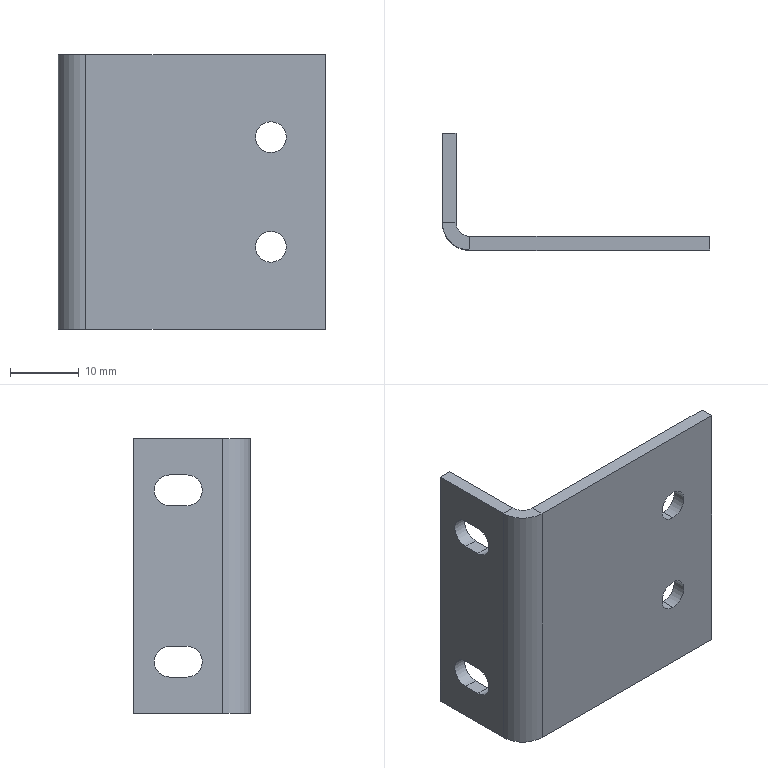Part | SolidWorks | features HoleWzd 2, FlatPattern 1, SMBaseFlange 1, SheetMetal 1 | 1 solid | 26 faces | box 39 x 17 x 40 mm | volume 4045 mm3 | plane 16 | cylinder 10 | commonest cylinder face diameters 4.5 x8 4 x1 8 x1
STEP:
#1=CARTESIAN_POINT('',(31.,-17.,9.75));
#2=VERTEX_POINT('',#1);
#3=CARTESIAN_POINT('',(31.,-17.,14.25));
#4=VERTEX_POINT('',#3);
#5=CARTESIAN_POINT('',(31.,-17.,12.));
#6=DIRECTION('',(0.,1.,0.));
#7=DIRECTION('',(0.,0.,1.));
#8=AXIS2_PLACEMENT_3D('',#5,#6,#7);
#9=CIRCLE('',#8,2.25);
#10=EDGE_CURVE('',#2,#4,#9,.T.);
#11=ORIENTED_EDGE('',*,*,#10,.F.);
#12=CARTESIAN_POINT('',(31.,-15.,9.75));
#13=VERTEX_POINT('',#12);
#14=CARTESIAN_POINT('',(31.,-15.,9.75));
#15=DIRECTION('',(0.,1.,0.));
#16=VECTOR('',#15,1000.);
#17=LINE('',#14,#16);
#18=EDGE_CURVE('',#2,#13,#17,.T.);
#19=ORIENTED_EDGE('',*,*,#18,.T.);
#20=CARTESIAN_POINT('',(31.,-15.,14.25));
#21=VERTEX_POINT('',#20);
#22=CARTESIAN_POINT('',(31.,-15.,12.));
#23=DIRECTION('',(0.,1.,0.));
#24=DIRECTION('',(0.,0.,1.));
#25=AXIS2_PLACEMENT_3D('',#22,#23,#24);
#26=CIRCLE('',#25,2.25);
#27=EDGE_CURVE('',#13,#21,#26,.T.);
#28=ORIENTED_EDGE('',*,*,#27,.T.);
#29=CARTESIAN_POINT('',(31.,-15.,14.25));
#30=DIRECTION('',(0.,1.,0.));
#31=VECTOR('',#30,1000.);
#32=LINE('',#29,#31);
#33=EDGE_CURVE('',#4,#21,#32,.T.);
#34=ORIENTED_EDGE('',*,*,#33,.F.);
#35=EDGE_LOOP('',(#11,#19,#28,#34));
#36=FACE_OUTER_BOUND('',#35,.T.);
#37=CARTESIAN_POINT('',(31.,-15.,12.));
#38=DIRECTION('',(0.,1.,0.));
#39=DIRECTION('',(0.,0.,1.));
#40=AXIS2_PLACEMENT_3D('',#37,#38,#39);
#41=CYLINDRICAL_SURFACE('',#40,2.25);
#42=ADVANCED_FACE('',(#36),#41,.F.);
#43=CARTESIAN_POINT('',(31.,-17.,25.75));
#44=VERTEX_POINT('',#43);
#45=CARTESIAN_POINT('',(31.,-17.,30.25));
#46=VERTEX_POINT('',#45);
#47=CARTESIAN_POINT('',(31.,-17.,28.));
#48=DIRECTION('',(0.,1.,0.));
#49=DIRECTION('',(0.,0.,1.));
#50=AXIS2_PLACEMENT_3D('',#47,#48,#49);
#51=CIRCLE('',#50,2.25);
#52=EDGE_CURVE('',#44,#46,#51,.T.);
#53=ORIENTED_EDGE('',*,*,#52,.F.);
#54=CARTESIAN_POINT('',(31.,-15.,25.75));
#55=VERTEX_POINT('',#54);
#56=CARTESIAN_POINT('',(31.,-15.,25.75));
#57=DIRECTION('',(0.,1.,0.));
#58=VECTOR('',#57,1000.);
#59=LINE('',#56,#58);
#60=EDGE_CURVE('',#44,#55,#59,.T.);
#61=ORIENTED_EDGE('',*,*,#60,.T.);
#62=CARTESIAN_POINT('',(31.,-15.,30.25));
#63=VERTEX_POINT('',#62);
#64=CARTESIAN_POINT('',(31.,-15.,28.));
#65=DIRECTION('',(0.,1.,0.));
#66=DIRECTION('',(0.,0.,1.));
#67=AXIS2_PLACEMENT_3D('',#64,#65,#66);
#68=CIRCLE('',#67,2.25);
#69=EDGE_CURVE('',#55,#63,#68,.T.);
#70=ORIENTED_EDGE('',*,*,#69,.T.);
#71=CARTESIAN_POINT('',(31.,-15.,30.25));
#72=DIRECTION('',(0.,1.,0.));
#73=VECTOR('',#72,1000.);
#74=LINE('',#71,#73);
#75=EDGE_CURVE('',#46,#63,#74,.T.);
#76=ORIENTED_EDGE('',*,*,#75,.F.);
#77=EDGE_LOOP('',(#53,#61,#70,#76));
#78=FACE_OUTER_BOUND('',#77,.T.);
#79=CARTESIAN_POINT('',(31.,-15.,28.));
#80=DIRECTION('',(0.,1.,0.));
#81=DIRECTION('',(0.,0.,1.));
#82=AXIS2_PLACEMENT_3D('',#79,#80,#81);
#83=CYLINDRICAL_SURFACE('',#82,2.25);
#84=ADVANCED_FACE('',(#78),#83,.F.);
#85=CARTESIAN_POINT('',(0.,-13.,40.));
#86=VERTEX_POINT('',#85);
#87=CARTESIAN_POINT('',(2.,-13.,40.));
#88=VERTEX_POINT('',#87);
#89=CARTESIAN_POINT('',(0.,-13.,40.));
#90=DIRECTION('',(1.,0.,0.));
#91=VECTOR('',#90,1000.);
#92=LINE('',#89,#91);
#93=EDGE_CURVE('',#86,#88,#92,.T.);
#94=ORIENTED_EDGE('',*,*,#93,.F.);
#95=CARTESIAN_POINT('',(4.,-17.,40.));
#96=VERTEX_POINT('',#95);
#97=CARTESIAN_POINT('',(4.,-13.,40.));
#98=DIRECTION('',(0.,0.,1.));
#99=DIRECTION('',(-1.,0.,0.));
#100=AXIS2_PLACEMENT_3D('',#97,#98,#99);
#101=CIRCLE('',#100,4.);
#102=EDGE_CURVE('',#86,#96,#101,.T.);
#103=ORIENTED_EDGE('',*,*,#102,.T.);
#104=CARTESIAN_POINT('',(4.,-15.,40.));
#105=VERTEX_POINT('',#104);
#106=CARTESIAN_POINT('',(4.,-15.,40.));
#107=DIRECTION('',(0.,-1.,0.));
#108=VECTOR('',#107,1000.);
#109=LINE('',#106,#108);
#110=EDGE_CURVE('',#105,#96,#109,.T.);
#111=ORIENTED_EDGE('',*,*,#110,.F.);
#112=CARTESIAN_POINT('',(4.,-13.,40.));
#113=DIRECTION('',(0.,0.,1.));
#114=DIRECTION('',(1.,0.,0.));
#115=AXIS2_PLACEMENT_3D('',#112,#113,#114);
#116=CIRCLE('',#115,2.);
#117=EDGE_CURVE('',#88,#105,#116,.T.);
#118=ORIENTED_EDGE('',*,*,#117,.F.);
#119=EDGE_LOOP('',(#94,#103,#111,#118));
#120=FACE_OUTER_BOUND('',#119,.T.);
#121=CARTESIAN_POINT('',(0.,-13.,40.));
#122=DIRECTION('',(0.,0.,1.));
#123=DIRECTION('',(1.,0.,0.));
#124=AXIS2_PLACEMENT_3D('',#121,#122,#123);
#125=PLANE('',#124);
#126=ADVANCED_FACE('',(#120),#125,.T.);
#127=CARTESIAN_POINT('',(0.,0.,40.));
#128=VERTEX_POINT('',#127);
#129=CARTESIAN_POINT('',(0.,0.,40.));
#130=DIRECTION('',(0.,-1.,0.));
#131=VECTOR('',#130,1000.);
#132=LINE('',#129,#131);
#133=EDGE_CURVE('',#128,#86,#132,.T.);
#134=ORIENTED_EDGE('',*,*,#133,.T.);
#135=ORIENTED_EDGE('',*,*,#93,.T.);
#136=CARTESIAN_POINT('',(2.,0.,40.));
#137=VERTEX_POINT('',#136);
#138=CARTESIAN_POINT('',(2.,0.,40.));
#139=DIRECTION('',(0.,-1.,0.));
#140=VECTOR('',#139,1000.);
#141=LINE('',#138,#140);
#142=EDGE_CURVE('',#137,#88,#141,.T.);
#143=ORIENTED_EDGE('',*,*,#142,.F.);
#144=CARTESIAN_POINT('',(0.,0.,40.));
#145=DIRECTION('',(1.,0.,0.));
#146=VECTOR('',#145,1000.);
#147=LINE('',#144,#146);
#148=EDGE_CURVE('',#128,#137,#147,.T.);
#149=ORIENTED_EDGE('',*,*,#148,.F.);
#150=EDGE_LOOP('',(#134,#135,#143,#149));
#151=FACE_OUTER_BOUND('',#150,.T.);
#152=CARTESIAN_POINT('',(4.,-15.,40.));
#153=DIRECTION('',(0.,0.,1.));
#154=DIRECTION('',(1.,0.,0.));
#155=AXIS2_PLACEMENT_3D('',#152,#153,#154);
#156=PLANE('',#155);
#157=ADVANCED_FACE('',(#151),#156,.T.);
#158=CARTESIAN_POINT('',(4.,-17.,0.));
#159=VERTEX_POINT('',#158);
#160=CARTESIAN_POINT('',(4.,-15.,0.));
#161=VERTEX_POINT('',#160);
#162=CARTESIAN_POINT('',(4.,-17.,0.));
#163=DIRECTION('',(0.,1.,0.));
#164=VECTOR('',#163,1000.);
#165=LINE('',#162,#164);
#166=EDGE_CURVE('',#159,#161,#165,.T.);
#167=ORIENTED_EDGE('',*,*,#166,.F.);
#168=CARTESIAN_POINT('',(0.,-13.,0.));
#169=VERTEX_POINT('',#168);
#170=CARTESIAN_POINT('',(4.,-13.,0.));
#171=DIRECTION('',(0.,0.,1.));
#172=DIRECTION('',(-1.,0.,0.));
#173=AXIS2_PLACEMENT_3D('',#170,#171,#172);
#174=CIRCLE('',#173,4.);
#175=EDGE_CURVE('',#169,#159,#174,.T.);
#176=ORIENTED_EDGE('',*,*,#175,.F.);
#177=CARTESIAN_POINT('',(2.,-13.,0.));
#178=VERTEX_POINT('',#177);
#179=CARTESIAN_POINT('',(2.,-13.,0.));
#180=DIRECTION('',(-1.,0.,0.));
#181=VECTOR('',#180,1000.);
#182=LINE('',#179,#181);
#183=EDGE_CURVE('',#178,#169,#182,.T.);
#184=ORIENTED_EDGE('',*,*,#183,.F.);
#185=CARTESIAN_POINT('',(4.,-13.,0.));
#186=DIRECTION('',(0.,0.,1.));
#187=DIRECTION('',(1.,0.,0.));
#188=AXIS2_PLACEMENT_3D('',#185,#186,#187);
#189=CIRCLE('',#188,2.);
#190=EDGE_CURVE('',#178,#161,#189,.T.);
#191=ORIENTED_EDGE('',*,*,#190,.T.);
#192=EDGE_LOOP('',(#167,#176,#184,#191));
#193=FACE_OUTER_BOUND('',#192,.T.);
#194=CARTESIAN_POINT('',(4.,-17.,0.));
#195=DIRECTION('',(0.,0.,-1.));
#196=DIRECTION('',(-1.,0.,0.));
#197=AXIS2_PLACEMENT_3D('',#194,#195,#196);
#198=PLANE('',#197);
#199=ADVANCED_FACE('',(#193),#198,.T.);
#200=CARTESIAN_POINT('',(39.,-17.,0.));
#201=VERTEX_POINT('',#200);
#202=CARTESIAN_POINT('',(0.,-17.,0.));
#203=DIRECTION('',(1.,0.,0.));
#204=VECTOR('',#203,1000.);
#205=LINE('',#202,#204);
#206=EDGE_CURVE('',#159,#201,#205,.T.);
#207=ORIENTED_EDGE('',*,*,#206,.F.);
#208=ORIENTED_EDGE('',*,*,#166,.T.);
#209=CARTESIAN_POINT('',(39.,-15.,0.));
#210=VERTEX_POINT('',#209);
#211=CARTESIAN_POINT('',(0.,-15.,0.));
#212=DIRECTION('',(1.,0.,0.));
#213=VECTOR('',#212,1000.);
#214=LINE('',#211,#213);
#215=EDGE_CURVE('',#161,#210,#214,.T.);
#216=ORIENTED_EDGE('',*,*,#215,.T.);
#217=CARTESIAN_POINT('',(39.,-15.,0.));
#218=DIRECTION('',(0.,-1.,0.));
#219=VECTOR('',#218,1000.);
#220=LINE('',#217,#219);
#221=EDGE_CURVE('',#210,#201,#220,.T.);
#222=ORIENTED_EDGE('',*,*,#221,.T.);
#223=EDGE_LOOP('',(#207,#208,#216,#222));
#224=FACE_OUTER_BOUND('',#223,.T.);
#225=CARTESIAN_POINT('',(2.,-13.,0.));
#226=DIRECTION('',(0.,0.,-1.));
#227=DIRECTION('',(-1.,0.,0.));
#228=AXIS2_PLACEMENT_3D('',#225,#226,#227);
#229=PLANE('',#228);
#230=ADVANCED_FACE('',(#224),#229,.T.);
#231=CARTESIAN_POINT('',(31.,-17.,12.));
#232=DIRECTION('',(0.,1.,0.));
#233=DIRECTION('',(0.,0.,1.));
#234=AXIS2_PLACEMENT_3D('',#231,#232,#233);
#235=CIRCLE('',#234,2.25);
#236=EDGE_CURVE('',#4,#2,#235,.T.);
#237=ORIENTED_EDGE('',*,*,#236,.T.);
#238=ORIENTED_EDGE('',*,*,#10,.T.);
#239=EDGE_LOOP('',(#237,#238));
#240=FACE_BOUND('',#239,.T.);
#241=CARTESIAN_POINT('',(31.,-17.,28.));
#242=DIRECTION('',(0.,1.,0.));
#243=DIRECTION('',(0.,0.,1.));
#244=AXIS2_PLACEMENT_3D('',#241,#242,#243);
#245=CIRCLE('',#244,2.25);
#246=EDGE_CURVE('',#46,#44,#245,.T.);
#247=ORIENTED_EDGE('',*,*,#246,.T.);
#248=ORIENTED_EDGE('',*,*,#52,.T.);
#249=EDGE_LOOP('',(#247,#248));
#250=FACE_BOUND('',#249,.T.);
#251=ORIENTED_EDGE('',*,*,#206,.T.);
#252=CARTESIAN_POINT('',(39.,-17.,40.));
#253=VERTEX_POINT('',#252);
#254=CARTESIAN_POINT('',(39.,-17.,40.));
#255=DIRECTION('',(0.,0.,-1.));
#256=VECTOR('',#255,1000.);
#257=LINE('',#254,#256);
#258=EDGE_CURVE('',#253,#201,#257,.T.);
#259=ORIENTED_EDGE('',*,*,#258,.F.);
#260=CARTESIAN_POINT('',(0.,-17.,40.));
#261=DIRECTION('',(1.,0.,0.));
#262=VECTOR('',#261,1000.);
#263=LINE('',#260,#262);
#264=EDGE_CURVE('',#96,#253,#263,.T.);
#265=ORIENTED_EDGE('',*,*,#264,.F.);
#266=CARTESIAN_POINT('',(4.,-17.,40.));
#267=DIRECTION('',(0.,0.,-1.));
#268=VECTOR('',#267,1000.);
#269=LINE('',#266,#268);
#270=EDGE_CURVE('',#96,#159,#269,.T.);
#271=ORIENTED_EDGE('',*,*,#270,.T.);
#272=EDGE_LOOP('',(#251,#259,#265,#271));
#273=FACE_OUTER_BOUND('',#272,.T.);
#274=CARTESIAN_POINT('',(0.,-17.,40.));
#275=DIRECTION('',(0.,1.,0.));
#276=DIRECTION('',(0.,0.,1.));
#277=AXIS2_PLACEMENT_3D('',#274,#275,#276);
#278=PLANE('',#277);
#279=ADVANCED_FACE('',(#240,#250,#273),#278,.F.);
#280=ORIENTED_EDGE('',*,*,#221,.F.);
#281=CARTESIAN_POINT('',(39.,-15.,40.));
#282=VERTEX_POINT('',#281);
#283=CARTESIAN_POINT('',(39.,-15.,40.));
#284=DIRECTION('',(0.,0.,-1.));
#285=VECTOR('',#284,1000.);
#286=LINE('',#283,#285);
#287=EDGE_CURVE('',#282,#210,#286,.T.);
#288=ORIENTED_EDGE('',*,*,#287,.F.);
#289=CARTESIAN_POINT('',(39.,-15.,40.));
#290=DIRECTION('',(0.,-1.,0.));
#291=VECTOR('',#290,1000.);
#292=LINE('',#289,#291);
#293=EDGE_CURVE('',#282,#253,#292,.T.);
#294=ORIENTED_EDGE('',*,*,#293,.T.);
#295=ORIENTED_EDGE('',*,*,#258,.T.);
#296=EDGE_LOOP('',(#280,#288,#294,#295));
#297=FACE_OUTER_BOUND('',#296,.T.);
#298=CARTESIAN_POINT('',(39.,-15.,40.));
#299=DIRECTION('',(1.,0.,0.));
#300=DIRECTION('',(0.,0.,-1.));
#301=AXIS2_PLACEMENT_3D('',#298,#299,#300);
#302=PLANE('',#301);
#303=ADVANCED_FACE('',(#297),#302,.T.);
#304=CARTESIAN_POINT('',(31.,-15.,12.));
#305=DIRECTION('',(0.,1.,0.));
#306=DIRECTION('',(0.,0.,1.));
#307=AXIS2_PLACEMENT_3D('',#304,#305,#306);
#308=CIRCLE('',#307,2.25);
#309=EDGE_CURVE('',#21,#13,#308,.T.);
#310=ORIENTED_EDGE('',*,*,#309,.F.);
#311=ORIENTED_EDGE('',*,*,#27,.F.);
#312=EDGE_LOOP('',(#310,#311));
#313=FACE_BOUND('',#312,.T.);
#314=CARTESIAN_POINT('',(31.,-15.,28.));
#315=DIRECTION('',(0.,1.,0.));
#316=DIRECTION('',(0.,0.,1.));
#317=AXIS2_PLACEMENT_3D('',#314,#315,#316);
#318=CIRCLE('',#317,2.25);
#319=EDGE_CURVE('',#63,#55,#318,.T.);
#320=ORIENTED_EDGE('',*,*,#319,.F.);
#321=ORIENTED_EDGE('',*,*,#69,.F.);
#322=EDGE_LOOP('',(#320,#321));
#323=FACE_BOUND('',#322,.T.);
#324=ORIENTED_EDGE('',*,*,#215,.F.);
#325=CARTESIAN_POINT('',(4.,-15.,40.));
#326=DIRECTION('',(0.,0.,-1.));
#327=VECTOR('',#326,1000.);
#328=LINE('',#325,#327);
#329=EDGE_CURVE('',#105,#161,#328,.T.);
#330=ORIENTED_EDGE('',*,*,#329,.F.);
#331=CARTESIAN_POINT('',(0.,-15.,40.));
#332=DIRECTION('',(1.,0.,0.));
#333=VECTOR('',#332,1000.);
#334=LINE('',#331,#333);
#335=EDGE_CURVE('',#105,#282,#334,.T.);
#336=ORIENTED_EDGE('',*,*,#335,.T.);
#337=ORIENTED_EDGE('',*,*,#287,.T.);
#338=EDGE_LOOP('',(#324,#330,#336,#337));
#339=FACE_OUTER_BOUND('',#338,.T.);
#340=CARTESIAN_POINT('',(0.,-15.,40.));
#341=DIRECTION('',(0.,1.,0.));
#342=DIRECTION('',(0.,0.,1.));
#343=AXIS2_PLACEMENT_3D('',#340,#341,#342);
#344=PLANE('',#343);
#345=ADVANCED_FACE('',(#313,#323,#339),#344,.T.);
#346=ORIENTED_EDGE('',*,*,#190,.F.);
#347=CARTESIAN_POINT('',(2.,-13.,40.));
#348=DIRECTION('',(0.,0.,-1.));
#349=VECTOR('',#348,1000.);
#350=LINE('',#347,#349);
#351=EDGE_CURVE('',#88,#178,#350,.T.);
#352=ORIENTED_EDGE('',*,*,#351,.F.);
#353=ORIENTED_EDGE('',*,*,#117,.T.);
#354=ORIENTED_EDGE('',*,*,#329,.T.);
#355=EDGE_LOOP('',(#346,#352,#353,#354));
#356=FACE_OUTER_BOUND('',#355,.T.);
#357=CARTESIAN_POINT('',(4.,-13.,40.));
#358=DIRECTION('',(0.,0.,-1.));
#359=DIRECTION('',(-1.,0.,0.));
#360=AXIS2_PLACEMENT_3D('',#357,#358,#359);
#361=CYLINDRICAL_SURFACE('',#360,2.);
#362=ADVANCED_FACE('',(#356),#361,.F.);
#363=CARTESIAN_POINT('',(2.,-7.75,5.25));
#364=VERTEX_POINT('',#363);
#365=CARTESIAN_POINT('',(2.,-5.25,5.25));
#366=VERTEX_POINT('',#365);
#367=CARTESIAN_POINT('',(2.,-7.75,5.25));
#368=DIRECTION('',(0.,1.,0.));
#369=VECTOR('',#368,1000.);
#370=LINE('',#367,#369);
#371=EDGE_CURVE('',#364,#366,#370,.T.);
#372=ORIENTED_EDGE('',*,*,#371,.F.);
#373=CARTESIAN_POINT('',(2.,-7.75,9.75));
#374=VERTEX_POINT('',#373);
#375=CARTESIAN_POINT('',(2.,-7.75,7.5));
#376=DIRECTION('',(1.,0.,0.));
#377=DIRECTION('',(0.,0.,-1.));
#378=AXIS2_PLACEMENT_3D('',#375,#376,#377);
#379=CIRCLE('',#378,2.25);
#380=EDGE_CURVE('',#374,#364,#379,.T.);
#381=ORIENTED_EDGE('',*,*,#380,.F.);
#382=CARTESIAN_POINT('',(2.,-5.25,9.75));
#383=VERTEX_POINT('',#382);
#384=CARTESIAN_POINT('',(2.,-7.75,9.75));
#385=DIRECTION('',(0.,1.,0.));
#386=VECTOR('',#385,1000.);
#387=LINE('',#384,#386);
#388=EDGE_CURVE('',#374,#383,#387,.T.);
#389=ORIENTED_EDGE('',*,*,#388,.T.);
#390=CARTESIAN_POINT('',(2.,-5.25,7.5));
#391=DIRECTION('',(1.,0.,0.));
#392=DIRECTION('',(0.,0.,-1.));
#393=AXIS2_PLACEMENT_3D('',#390,#391,#392);
#394=CIRCLE('',#393,2.25);
#395=EDGE_CURVE('',#366,#383,#394,.T.);
#396=ORIENTED_EDGE('',*,*,#395,.F.);
#397=EDGE_LOOP('',(#372,#381,#389,#396));
#398=FACE_BOUND('',#397,.T.);
#399=CARTESIAN_POINT('',(2.,-5.25,30.25));
#400=VERTEX_POINT('',#399);
#401=CARTESIAN_POINT('',(2.,-5.25,34.75));
#402=VERTEX_POINT('',#401);
#403=CARTESIAN_POINT('',(2.,-5.25,32.5));
#404=DIRECTION('',(1.,0.,0.));
#405=DIRECTION('',(0.,0.,-1.));
#406=AXIS2_PLACEMENT_3D('',#403,#404,#405);
#407=CIRCLE('',#406,2.25);
#408=EDGE_CURVE('',#400,#402,#407,.T.);
#409=ORIENTED_EDGE('',*,*,#408,.F.);
#410=CARTESIAN_POINT('',(2.,-7.75,30.25));
#411=VERTEX_POINT('',#410);
#412=CARTESIAN_POINT('',(2.,-7.75,30.25));
#413=DIRECTION('',(0.,1.,0.));
#414=VECTOR('',#413,1000.);
#415=LINE('',#412,#414);
#416=EDGE_CURVE('',#411,#400,#415,.T.);
#417=ORIENTED_EDGE('',*,*,#416,.F.);
#418=CARTESIAN_POINT('',(2.,-7.75,34.75));
#419=VERTEX_POINT('',#418);
#420=CARTESIAN_POINT('',(2.,-7.75,32.5));
#421=DIRECTION('',(1.,0.,0.));
#422=DIRECTION('',(0.,0.,-1.));
#423=AXIS2_PLACEMENT_3D('',#420,#421,#422);
#424=CIRCLE('',#423,2.25);
#425=EDGE_CURVE('',#419,#411,#424,.T.);
#426=ORIENTED_EDGE('',*,*,#425,.F.);
#427=CARTESIAN_POINT('',(2.,-7.75,34.75));
#428=DIRECTION('',(0.,1.,0.));
#429=VECTOR('',#428,1000.);
#430=LINE('',#427,#429);
#431=EDGE_CURVE('',#419,#402,#430,.T.);
#432=ORIENTED_EDGE('',*,*,#431,.T.);
#433=EDGE_LOOP('',(#409,#417,#426,#432));
#434=FACE_BOUND('',#433,.T.);
#435=CARTESIAN_POINT('',(2.,0.,0.));
#436=VERTEX_POINT('',#435);
#437=CARTESIAN_POINT('',(2.,0.,0.));
#438=DIRECTION('',(0.,-1.,0.));
#439=VECTOR('',#438,1000.);
#440=LINE('',#437,#439);
#441=EDGE_CURVE('',#436,#178,#440,.T.);
#442=ORIENTED_EDGE('',*,*,#441,.F.);
#443=CARTESIAN_POINT('',(2.,0.,40.));
#444=DIRECTION('',(0.,0.,-1.));
#445=VECTOR('',#444,1000.);
#446=LINE('',#443,#445);
#447=EDGE_CURVE('',#137,#436,#446,.T.);
#448=ORIENTED_EDGE('',*,*,#447,.F.);
#449=ORIENTED_EDGE('',*,*,#142,.T.);
#450=ORIENTED_EDGE('',*,*,#351,.T.);
#451=EDGE_LOOP('',(#442,#448,#449,#450));
#452=FACE_OUTER_BOUND('',#451,.T.);
#453=CARTESIAN_POINT('',(2.,0.,40.));
#454=DIRECTION('',(1.,0.,0.));
#455=DIRECTION('',(0.,1.,0.));
#456=AXIS2_PLACEMENT_3D('',#453,#454,#455);
#457=PLANE('',#456);
#458=ADVANCED_FACE('',(#398,#434,#452),#457,.T.);
#459=CARTESIAN_POINT('',(0.,0.,0.));
#460=VERTEX_POINT('',#459);
#461=CARTESIAN_POINT('',(0.,0.,0.));
#462=DIRECTION('',(1.,0.,0.));
#463=VECTOR('',#462,1000.);
#464=LINE('',#461,#463);
#465=EDGE_CURVE('',#460,#436,#464,.T.);
#466=ORIENTED_EDGE('',*,*,#465,.F.);
#467=CARTESIAN_POINT('',(0.,0.,40.));
#468=DIRECTION('',(0.,0.,-1.));
#469=VECTOR('',#468,1000.);
#470=LINE('',#467,#469);
#471=EDGE_CURVE('',#128,#460,#470,.T.);
#472=ORIENTED_EDGE('',*,*,#471,.F.);
#473=ORIENTED_EDGE('',*,*,#148,.T.);
#474=ORIENTED_EDGE('',*,*,#447,.T.);
#475=EDGE_LOOP('',(#466,#472,#473,#474));
#476=FACE_OUTER_BOUND('',#475,.T.);
#477=CARTESIAN_POINT('',(0.,0.,40.));
#478=DIRECTION('',(0.,1.,0.));
#479=DIRECTION('',(-1.,0.,0.));
#480=AXIS2_PLACEMENT_3D('',#477,#478,#479);
#481=PLANE('',#480);
#482=ADVANCED_FACE('',(#476),#481,.T.);
#483=CARTESIAN_POINT('',(0.,-5.25,9.75));
#484=VERTEX_POINT('',#483);
#485=CARTESIAN_POINT('',(0.,-7.75,9.75));
#486=VERTEX_POINT('',#485);
#487=CARTESIAN_POINT('',(0.,0.,9.75));
#488=DIRECTION('',(0.,-1.,0.));
#489=VECTOR('',#488,1000.);
#490=LINE('',#487,#489);
#491=EDGE_CURVE('',#484,#486,#490,.T.);
#492=ORIENTED_EDGE('',*,*,#491,.T.);
#493=CARTESIAN_POINT('',(0.,-7.75,5.25));
#494=VERTEX_POINT('',#493);
#495=CARTESIAN_POINT('',(0.,-7.75,7.5));
#496=DIRECTION('',(1.,0.,0.));
#497=DIRECTION('',(0.,1.,0.));
#498=AXIS2_PLACEMENT_3D('',#495,#496,#497);
#499=CIRCLE('',#498,2.25);
#500=EDGE_CURVE('',#486,#494,#499,.T.);
#501=ORIENTED_EDGE('',*,*,#500,.T.);
#502=CARTESIAN_POINT('',(0.,-5.25,5.25));
#503=VERTEX_POINT('',#502);
#504=CARTESIAN_POINT('',(0.,0.,5.25));
#505=DIRECTION('',(0.,1.,0.));
#506=VECTOR('',#505,1000.);
#507=LINE('',#504,#506);
#508=EDGE_CURVE('',#494,#503,#507,.T.);
#509=ORIENTED_EDGE('',*,*,#508,.T.);
#510=CARTESIAN_POINT('',(0.,-5.25,7.5));
#511=DIRECTION('',(1.,0.,0.));
#512=DIRECTION('',(0.,1.,0.));
#513=AXIS2_PLACEMENT_3D('',#510,#511,#512);
#514=CIRCLE('',#513,2.25);
#515=EDGE_CURVE('',#503,#484,#514,.T.);
#516=ORIENTED_EDGE('',*,*,#515,.T.);
#517=EDGE_LOOP('',(#492,#501,#509,#516));
#518=FACE_BOUND('',#517,.T.);
#519=CARTESIAN_POINT('',(0.,-5.25,34.75));
#520=VERTEX_POINT('',#519);
#521=CARTESIAN_POINT('',(0.,-7.75,34.75));
#522=VERTEX_POINT('',#521);
#523=CARTESIAN_POINT('',(0.,0.,34.75));
#524=DIRECTION('',(0.,-1.,0.));
#525=VECTOR('',#524,1000.);
#526=LINE('',#523,#525);
#527=EDGE_CURVE('',#520,#522,#526,.T.);
#528=ORIENTED_EDGE('',*,*,#527,.T.);
#529=CARTESIAN_POINT('',(0.,-7.75,30.25));
#530=VERTEX_POINT('',#529);
#531=CARTESIAN_POINT('',(0.,-7.75,32.5));
#532=DIRECTION('',(1.,0.,0.));
#533=DIRECTION('',(0.,1.,0.));
#534=AXIS2_PLACEMENT_3D('',#531,#532,#533);
#535=CIRCLE('',#534,2.25);
#536=EDGE_CURVE('',#522,#530,#535,.T.);
#537=ORIENTED_EDGE('',*,*,#536,.T.);
#538=CARTESIAN_POINT('',(0.,-5.25,30.25));
#539=VERTEX_POINT('',#538);
#540=CARTESIAN_POINT('',(0.,0.,30.25));
#541=DIRECTION('',(0.,1.,0.));
#542=VECTOR('',#541,1000.);
#543=LINE('',#540,#542);
#544=EDGE_CURVE('',#530,#539,#543,.T.);
#545=ORIENTED_EDGE('',*,*,#544,.T.);
#546=CARTESIAN_POINT('',(0.,-5.25,32.5));
#547=DIRECTION('',(1.,0.,0.));
#548=DIRECTION('',(0.,1.,0.));
#549=AXIS2_PLACEMENT_3D('',#546,#547,#548);
#550=CIRCLE('',#549,2.25);
#551=EDGE_CURVE('',#539,#520,#550,.T.);
#552=ORIENTED_EDGE('',*,*,#551,.T.);
#553=EDGE_LOOP('',(#528,#537,#545,#552));
#554=FACE_BOUND('',#553,.T.);
#555=CARTESIAN_POINT('',(0.,0.,0.));
#556=DIRECTION('',(0.,-1.,0.));
#557=VECTOR('',#556,1000.);
#558=LINE('',#555,#557);
#559=EDGE_CURVE('',#460,#169,#558,.T.);
#560=ORIENTED_EDGE('',*,*,#559,.T.);
#561=CARTESIAN_POINT('',(0.,-13.,40.));
#562=DIRECTION('',(0.,0.,-1.));
#563=VECTOR('',#562,1000.);
#564=LINE('',#561,#563);
#565=EDGE_CURVE('',#86,#169,#564,.T.);
#566=ORIENTED_EDGE('',*,*,#565,.F.);
#567=ORIENTED_EDGE('',*,*,#133,.F.);
#568=ORIENTED_EDGE('',*,*,#471,.T.);
#569=EDGE_LOOP('',(#560,#566,#567,#568));
#570=FACE_OUTER_BOUND('',#569,.T.);
#571=CARTESIAN_POINT('',(0.,0.,40.));
#572=DIRECTION('',(1.,0.,0.));
#573=DIRECTION('',(0.,1.,0.));
#574=AXIS2_PLACEMENT_3D('',#571,#572,#573);
#575=PLANE('',#574);
#576=ADVANCED_FACE('',(#518,#554,#570),#575,.F.);
#577=ORIENTED_EDGE('',*,*,#175,.T.);
#578=ORIENTED_EDGE('',*,*,#270,.F.);
#579=ORIENTED_EDGE('',*,*,#102,.F.);
#580=ORIENTED_EDGE('',*,*,#565,.T.);
#581=EDGE_LOOP('',(#577,#578,#579,#580));
#582=FACE_OUTER_BOUND('',#581,.T.);
#583=CARTESIAN_POINT('',(4.,-13.,40.));
#584=DIRECTION('',(0.,0.,-1.));
#585=DIRECTION('',(-1.,0.,0.));
#586=AXIS2_PLACEMENT_3D('',#583,#584,#585);
#587=CYLINDRICAL_SURFACE('',#586,4.);
#588=ADVANCED_FACE('',(#582),#587,.T.);
#589=ORIENTED_EDGE('',*,*,#264,.T.);
#590=ORIENTED_EDGE('',*,*,#293,.F.);
#591=ORIENTED_EDGE('',*,*,#335,.F.);
#592=ORIENTED_EDGE('',*,*,#110,.T.);
#593=EDGE_LOOP('',(#589,#590,#591,#592));
#594=FACE_OUTER_BOUND('',#593,.T.);
#595=CARTESIAN_POINT('',(4.,-13.,40.));
#596=DIRECTION('',(0.,0.,1.));
#597=DIRECTION('',(1.,0.,0.));
#598=AXIS2_PLACEMENT_3D('',#595,#596,#597);
#599=PLANE('',#598);
#600=ADVANCED_FACE('',(#594),#599,.T.);
#601=ORIENTED_EDGE('',*,*,#441,.T.);
#602=ORIENTED_EDGE('',*,*,#183,.T.);
#603=ORIENTED_EDGE('',*,*,#559,.F.);
#604=ORIENTED_EDGE('',*,*,#465,.T.);
#605=EDGE_LOOP('',(#601,#602,#603,#604));
#606=FACE_OUTER_BOUND('',#605,.T.);
#607=CARTESIAN_POINT('',(4.,-13.,0.));
#608=DIRECTION('',(0.,0.,1.));
#609=DIRECTION('',(1.,0.,0.));
#610=AXIS2_PLACEMENT_3D('',#607,#608,#609);
#611=PLANE('',#610);
#612=ADVANCED_FACE('',(#606),#611,.F.);
#613=ORIENTED_EDGE('',*,*,#60,.F.);
#614=ORIENTED_EDGE('',*,*,#246,.F.);
#615=ORIENTED_EDGE('',*,*,#75,.T.);
#616=ORIENTED_EDGE('',*,*,#319,.T.);
#617=EDGE_LOOP('',(#613,#614,#615,#616));
#618=FACE_OUTER_BOUND('',#617,.T.);
#619=CARTESIAN_POINT('',(31.,-15.,28.));
#620=DIRECTION('',(0.,1.,0.));
#621=DIRECTION('',(0.,0.,1.));
#622=AXIS2_PLACEMENT_3D('',#619,#620,#621);
#623=CYLINDRICAL_SURFACE('',#622,2.25);
#624=ADVANCED_FACE('',(#618),#623,.F.);
#625=ORIENTED_EDGE('',*,*,#18,.F.);
#626=ORIENTED_EDGE('',*,*,#236,.F.);
#627=ORIENTED_EDGE('',*,*,#33,.T.);
#628=ORIENTED_EDGE('',*,*,#309,.T.);
#629=EDGE_LOOP('',(#625,#626,#627,#628));
#630=FACE_OUTER_BOUND('',#629,.T.);
#631=CARTESIAN_POINT('',(31.,-15.,12.));
#632=DIRECTION('',(0.,1.,0.));
#633=DIRECTION('',(0.,0.,1.));
#634=AXIS2_PLACEMENT_3D('',#631,#632,#633);
#635=CYLINDRICAL_SURFACE('',#634,2.25);
#636=ADVANCED_FACE('',(#630),#635,.F.);
#637=CARTESIAN_POINT('',(2.,-7.75,34.75));
#638=DIRECTION('',(-1.,0.,0.));
#639=VECTOR('',#638,1000.);
#640=LINE('',#637,#639);
#641=EDGE_CURVE('',#419,#522,#640,.T.);
#642=ORIENTED_EDGE('',*,*,#641,.F.);
#643=ORIENTED_EDGE('',*,*,#425,.T.);
#644=CARTESIAN_POINT('',(2.,-7.75,30.25));
#645=DIRECTION('',(1.,0.,0.));
#646=VECTOR('',#645,1000.);
#647=LINE('',#644,#646);
#648=EDGE_CURVE('',#530,#411,#647,.T.);
#649=ORIENTED_EDGE('',*,*,#648,.F.);
#650=ORIENTED_EDGE('',*,*,#536,.F.);
#651=EDGE_LOOP('',(#642,#643,#649,#650));
#652=FACE_OUTER_BOUND('',#651,.T.);
#653=CARTESIAN_POINT('',(2.,-7.75,32.5));
#654=DIRECTION('',(1.,0.,0.));
#655=DIRECTION('',(0.,0.,-1.));
#656=AXIS2_PLACEMENT_3D('',#653,#654,#655);
#657=CYLINDRICAL_SURFACE('',#656,2.25);
#658=ADVANCED_FACE('',(#652),#657,.F.);
#659=CARTESIAN_POINT('',(2.,-5.25,30.25));
#660=DIRECTION('',(-1.,0.,0.));
#661=VECTOR('',#660,1000.);
#662=LINE('',#659,#661);
#663=EDGE_CURVE('',#400,#539,#662,.T.);
#664=ORIENTED_EDGE('',*,*,#663,.F.);
#665=ORIENTED_EDGE('',*,*,#408,.T.);
#666=CARTESIAN_POINT('',(2.,-5.25,34.75));
#667=DIRECTION('',(1.,0.,0.));
#668=VECTOR('',#667,1000.);
#669=LINE('',#666,#668);
#670=EDGE_CURVE('',#520,#402,#669,.T.);
#671=ORIENTED_EDGE('',*,*,#670,.F.);
#672=ORIENTED_EDGE('',*,*,#551,.F.);
#673=EDGE_LOOP('',(#664,#665,#671,#672));
#674=FACE_OUTER_BOUND('',#673,.T.);
#675=CARTESIAN_POINT('',(2.,-5.25,32.5));
#676=DIRECTION('',(1.,0.,0.));
#677=DIRECTION('',(0.,0.,-1.));
#678=AXIS2_PLACEMENT_3D('',#675,#676,#677);
#679=CYLINDRICAL_SURFACE('',#678,2.25);
#680=ADVANCED_FACE('',(#674),#679,.F.);
#681=ORIENTED_EDGE('',*,*,#648,.T.);
#682=ORIENTED_EDGE('',*,*,#416,.T.);
#683=ORIENTED_EDGE('',*,*,#663,.T.);
#684=ORIENTED_EDGE('',*,*,#544,.F.);
#685=EDGE_LOOP('',(#681,#682,#683,#684));
#686=FACE_OUTER_BOUND('',#685,.T.);
#687=CARTESIAN_POINT('',(2.,-7.75,30.25));
#688=DIRECTION('',(0.,0.,-1.));
#689=DIRECTION('',(-1.,0.,0.));
#690=AXIS2_PLACEMENT_3D('',#687,#688,#689);
#691=PLANE('',#690);
#692=ADVANCED_FACE('',(#686),#691,.F.);
#693=ORIENTED_EDGE('',*,*,#670,.T.);
#694=ORIENTED_EDGE('',*,*,#431,.F.);
#695=ORIENTED_EDGE('',*,*,#641,.T.);
#696=ORIENTED_EDGE('',*,*,#527,.F.);
#697=EDGE_LOOP('',(#693,#694,#695,#696));
#698=FACE_OUTER_BOUND('',#697,.T.);
#699=CARTESIAN_POINT('',(2.,-7.75,34.75));
#700=DIRECTION('',(0.,0.,1.));
#701=DIRECTION('',(1.,0.,0.));
#702=AXIS2_PLACEMENT_3D('',#699,#700,#701);
#703=PLANE('',#702);
#704=ADVANCED_FACE('',(#698),#703,.F.);
#705=CARTESIAN_POINT('',(2.,-7.75,5.25));
#706=DIRECTION('',(1.,0.,0.));
#707=VECTOR('',#706,1000.);
#708=LINE('',#705,#707);
#709=EDGE_CURVE('',#494,#364,#708,.T.);
#710=ORIENTED_EDGE('',*,*,#709,.T.);
#711=ORIENTED_EDGE('',*,*,#371,.T.);
#712=CARTESIAN_POINT('',(2.,-5.25,5.25));
#713=DIRECTION('',(-1.,0.,0.));
#714=VECTOR('',#713,1000.);
#715=LINE('',#712,#714);
#716=EDGE_CURVE('',#366,#503,#715,.T.);
#717=ORIENTED_EDGE('',*,*,#716,.T.);
#718=ORIENTED_EDGE('',*,*,#508,.F.);
#719=EDGE_LOOP('',(#710,#711,#717,#718));
#720=FACE_OUTER_BOUND('',#719,.T.);
#721=CARTESIAN_POINT('',(2.,-7.75,5.25));
#722=DIRECTION('',(0.,0.,-1.));
#723=DIRECTION('',(-1.,0.,0.));
#724=AXIS2_PLACEMENT_3D('',#721,#722,#723);
#725=PLANE('',#724);
#726=ADVANCED_FACE('',(#720),#725,.F.);
#727=ORIENTED_EDGE('',*,*,#716,.F.);
#728=ORIENTED_EDGE('',*,*,#395,.T.);
#729=CARTESIAN_POINT('',(2.,-5.25,9.75));
#730=DIRECTION('',(1.,0.,0.));
#731=VECTOR('',#730,1000.);
#732=LINE('',#729,#731);
#733=EDGE_CURVE('',#484,#383,#732,.T.);
#734=ORIENTED_EDGE('',*,*,#733,.F.);
#735=ORIENTED_EDGE('',*,*,#515,.F.);
#736=EDGE_LOOP('',(#727,#728,#734,#735));
#737=FACE_OUTER_BOUND('',#736,.T.);
#738=CARTESIAN_POINT('',(2.,-5.25,7.5));
#739=DIRECTION('',(1.,0.,0.));
#740=DIRECTION('',(0.,0.,-1.));
#741=AXIS2_PLACEMENT_3D('',#738,#739,#740);
#742=CYLINDRICAL_SURFACE('',#741,2.25);
#743=ADVANCED_FACE('',(#737),#742,.F.);
#744=CARTESIAN_POINT('',(2.,-7.75,9.75));
#745=DIRECTION('',(-1.,0.,0.));
#746=VECTOR('',#745,1000.);
#747=LINE('',#744,#746);
#748=EDGE_CURVE('',#374,#486,#747,.T.);
#749=ORIENTED_EDGE('',*,*,#748,.F.);
#750=ORIENTED_EDGE('',*,*,#380,.T.);
#751=ORIENTED_EDGE('',*,*,#709,.F.);
#752=ORIENTED_EDGE('',*,*,#500,.F.);
#753=EDGE_LOOP('',(#749,#750,#751,#752));
#754=FACE_OUTER_BOUND('',#753,.T.);
#755=CARTESIAN_POINT('',(2.,-7.75,7.5));
#756=DIRECTION('',(1.,0.,0.));
#757=DIRECTION('',(0.,0.,-1.));
#758=AXIS2_PLACEMENT_3D('',#755,#756,#757);
#759=CYLINDRICAL_SURFACE('',#758,2.25);
#760=ADVANCED_FACE('',(#754),#759,.F.);
#761=ORIENTED_EDGE('',*,*,#733,.T.);
#762=ORIENTED_EDGE('',*,*,#388,.F.);
#763=ORIENTED_EDGE('',*,*,#748,.T.);
#764=ORIENTED_EDGE('',*,*,#491,.F.);
#765=EDGE_LOOP('',(#761,#762,#763,#764));
#766=FACE_OUTER_BOUND('',#765,.T.);
#767=CARTESIAN_POINT('',(2.,-7.75,9.75));
#768=DIRECTION('',(0.,0.,1.));
#769=DIRECTION('',(1.,0.,0.));
#770=AXIS2_PLACEMENT_3D('',#767,#768,#769);
#771=PLANE('',#770);
#772=ADVANCED_FACE('',(#766),#771,.F.);
#773=CLOSED_SHELL('',(#42,#84,#126,#157,#199,#230,#279,#303,#345,#362,#458,#482,#576,#588,#600,#612,#624,#636,#658,#680,#692,#704,#726,#743,#760,#772));
#774=MANIFOLD_SOLID_BREP('',#773);
#775=CARTESIAN_POINT('',(0.,0.,0.));
#776=DIRECTION('',(0.,0.,1.));
#777=DIRECTION('',(1.,0.,0.));
#778=AXIS2_PLACEMENT_3D('',#775,#776,#777);
#779=(LENGTH_UNIT()NAMED_UNIT(*)SI_UNIT(.MILLI.,.METRE.));
#780=UNCERTAINTY_MEASURE_WITH_UNIT(LENGTH_MEASURE(0.00001),#779,'','');
#781=(NAMED_UNIT(*)PLANE_ANGLE_UNIT()SI_UNIT($,.RADIAN.));
#782=(NAMED_UNIT(*)SI_UNIT($,.STERADIAN.)SOLID_ANGLE_UNIT());
#783=(GEOMETRIC_REPRESENTATION_CONTEXT(3)GLOBAL_UNCERTAINTY_ASSIGNED_CONTEXT((#780))GLOBAL_UNIT_ASSIGNED_CONTEXT((#779,#781,#782))REPRESENTATION_CONTEXT('',''));
#784=ADVANCED_BREP_SHAPE_REPRESENTATION('',(#774,#778),#783);